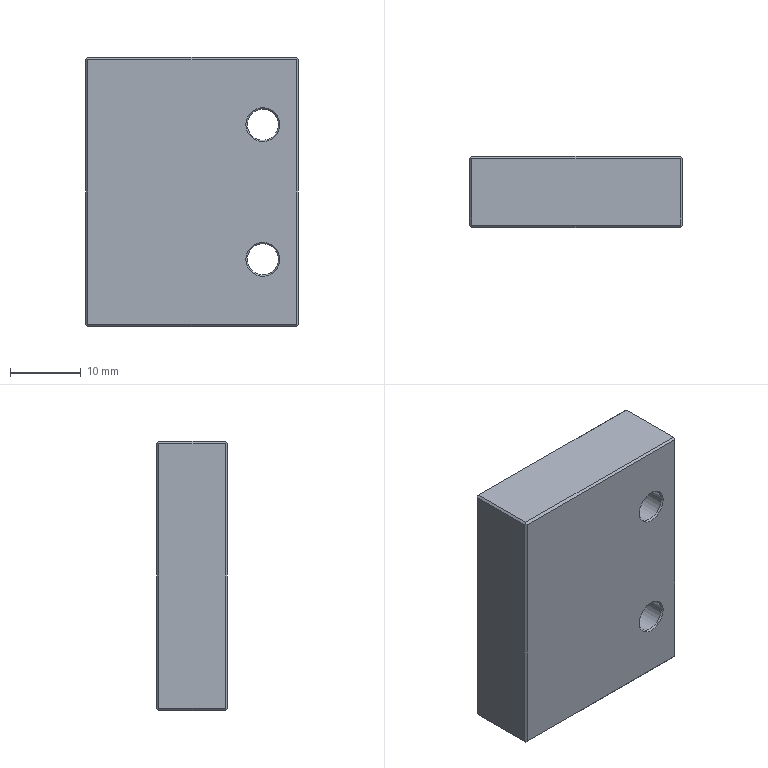Part | NX | 1 solid | 42 faces | box 30 x 10 x 38 mm | volume 10990 mm3 | plane 18 | cylinder 12 | cone 12 | commonest cylinder face diameters 2.5 x8 4.4 x4
STEP:
#1=CARTESIAN_POINT('',(-28.3,-35.,40.2));
#2=VERTEX_POINT('',#1);
#3=CARTESIAN_POINT('',(-28.3,-35.,2.8));
#4=VERTEX_POINT('',#3);
#5=CARTESIAN_POINT('',(-28.3,-35.,21.5));
#6=DIRECTION('',(0.,0.,-1.));
#7=VECTOR('',#6,1000.);
#8=LINE('',#5,#7);
#9=EDGE_CURVE('',#2,#4,#8,.T.);
#10=ORIENTED_EDGE('',*,*,#9,.F.);
#11=CARTESIAN_POINT('',(-57.7,-35.,40.2));
#12=VERTEX_POINT('',#11);
#13=CARTESIAN_POINT('',(-43.,-35.,40.2));
#14=DIRECTION('',(-1.,0.,0.));
#15=VECTOR('',#14,1000.);
#16=LINE('',#13,#15);
#17=EDGE_CURVE('',#2,#12,#16,.T.);
#18=ORIENTED_EDGE('',*,*,#17,.T.);
#19=CARTESIAN_POINT('',(-57.7,-35.,2.8));
#20=VERTEX_POINT('',#19);
#21=CARTESIAN_POINT('',(-57.7,-35.,21.5));
#22=DIRECTION('',(0.,0.,-1.));
#23=VECTOR('',#22,1000.);
#24=LINE('',#21,#23);
#25=EDGE_CURVE('',#12,#20,#24,.T.);
#26=ORIENTED_EDGE('',*,*,#25,.T.);
#27=CARTESIAN_POINT('',(-43.,-35.,2.8));
#28=DIRECTION('',(1.,0.,0.));
#29=VECTOR('',#28,1000.);
#30=LINE('',#27,#29);
#31=EDGE_CURVE('',#20,#4,#30,.T.);
#32=ORIENTED_EDGE('',*,*,#31,.T.);
#33=EDGE_LOOP('',(#10,#18,#26,#32));
#34=FACE_BOUND('',#33,.T.);
#35=CARTESIAN_POINT('',(-30.6,-35.,31.));
#36=VERTEX_POINT('',#35);
#37=CARTESIAN_POINT('',(-35.4,-35.,31.));
#38=VERTEX_POINT('',#37);
#39=CARTESIAN_POINT('',(-33.,-35.,31.));
#40=DIRECTION('',(0.,-1.,0.));
#41=DIRECTION('',(-1.,0.,0.));
#42=AXIS2_PLACEMENT_3D('',#39,#40,#41);
#43=CIRCLE('',#42,2.4);
#44=EDGE_CURVE('',#36,#38,#43,.T.);
#45=ORIENTED_EDGE('',*,*,#44,.F.);
#46=CARTESIAN_POINT('',(-33.,-35.,31.));
#47=DIRECTION('',(0.,-1.,0.));
#48=DIRECTION('',(-1.,0.,0.));
#49=AXIS2_PLACEMENT_3D('',#46,#47,#48);
#50=CIRCLE('',#49,2.4);
#51=EDGE_CURVE('',#38,#36,#50,.T.);
#52=ORIENTED_EDGE('',*,*,#51,.F.);
#53=EDGE_LOOP('',(#45,#52));
#54=FACE_BOUND('',#53,.T.);
#55=CARTESIAN_POINT('',(-30.6,-35.,12.));
#56=VERTEX_POINT('',#55);
#57=CARTESIAN_POINT('',(-35.4,-35.,12.));
#58=VERTEX_POINT('',#57);
#59=CARTESIAN_POINT('',(-33.,-35.,12.));
#60=DIRECTION('',(0.,-1.,0.));
#61=DIRECTION('',(-1.,0.,0.));
#62=AXIS2_PLACEMENT_3D('',#59,#60,#61);
#63=CIRCLE('',#62,2.4);
#64=EDGE_CURVE('',#56,#58,#63,.T.);
#65=ORIENTED_EDGE('',*,*,#64,.F.);
#66=CARTESIAN_POINT('',(-33.,-35.,12.));
#67=DIRECTION('',(0.,-1.,0.));
#68=DIRECTION('',(-1.,0.,0.));
#69=AXIS2_PLACEMENT_3D('',#66,#67,#68);
#70=CIRCLE('',#69,2.4);
#71=EDGE_CURVE('',#58,#56,#70,.T.);
#72=ORIENTED_EDGE('',*,*,#71,.F.);
#73=EDGE_LOOP('',(#65,#72));
#74=FACE_BOUND('',#73,.T.);
#75=CARTESIAN_POINT('',(0.,-35.,0.));
#76=DIRECTION('',(0.,1.,0.));
#77=DIRECTION('',(1.,0.,0.));
#78=AXIS2_PLACEMENT_3D('',#75,#76,#77);
#79=PLANE('',#78);
#80=ADVANCED_FACE('',(#34,#54,#74),#79,.F.);
#81=CARTESIAN_POINT('',(-58.,-25.3,2.8));
#82=VERTEX_POINT('',#81);
#83=CARTESIAN_POINT('',(-58.,-25.3,40.2));
#84=VERTEX_POINT('',#83);
#85=CARTESIAN_POINT('',(-58.,-25.3,21.5));
#86=DIRECTION('',(0.,0.,1.));
#87=VECTOR('',#86,1000.);
#88=LINE('',#85,#87);
#89=EDGE_CURVE('',#82,#84,#88,.T.);
#90=ORIENTED_EDGE('',*,*,#89,.F.);
#91=CARTESIAN_POINT('',(-58.,-34.7,2.8));
#92=VERTEX_POINT('',#91);
#93=CARTESIAN_POINT('',(-58.,-30.,2.8));
#94=DIRECTION('',(0.,1.,0.));
#95=VECTOR('',#94,1000.);
#96=LINE('',#93,#95);
#97=EDGE_CURVE('',#92,#82,#96,.T.);
#98=ORIENTED_EDGE('',*,*,#97,.F.);
#99=CARTESIAN_POINT('',(-58.,-34.7,40.2));
#100=VERTEX_POINT('',#99);
#101=CARTESIAN_POINT('',(-58.,-34.7,21.5));
#102=DIRECTION('',(0.,0.,-1.));
#103=VECTOR('',#102,1000.);
#104=LINE('',#101,#103);
#105=EDGE_CURVE('',#100,#92,#104,.T.);
#106=ORIENTED_EDGE('',*,*,#105,.F.);
#107=CARTESIAN_POINT('',(-58.,-30.,40.2));
#108=DIRECTION('',(0.,-1.,0.));
#109=VECTOR('',#108,1000.);
#110=LINE('',#107,#109);
#111=EDGE_CURVE('',#84,#100,#110,.T.);
#112=ORIENTED_EDGE('',*,*,#111,.F.);
#113=EDGE_LOOP('',(#90,#98,#106,#112));
#114=FACE_BOUND('',#113,.T.);
#115=CARTESIAN_POINT('',(-58.,0.,0.));
#116=DIRECTION('',(1.,0.,0.));
#117=DIRECTION('',(0.,1.,0.));
#118=AXIS2_PLACEMENT_3D('',#115,#116,#117);
#119=PLANE('',#118);
#120=ADVANCED_FACE('',(#114),#119,.F.);
#121=CARTESIAN_POINT('',(-28.3,-25.,2.8));
#122=VERTEX_POINT('',#121);
#123=CARTESIAN_POINT('',(-28.3,-25.,40.2));
#124=VERTEX_POINT('',#123);
#125=CARTESIAN_POINT('',(-28.3,-25.,21.5));
#126=DIRECTION('',(0.,0.,1.));
#127=VECTOR('',#126,1000.);
#128=LINE('',#125,#127);
#129=EDGE_CURVE('',#122,#124,#128,.T.);
#130=ORIENTED_EDGE('',*,*,#129,.F.);
#131=CARTESIAN_POINT('',(-57.7,-25.,2.8));
#132=VERTEX_POINT('',#131);
#133=CARTESIAN_POINT('',(-43.,-25.,2.8));
#134=DIRECTION('',(1.,0.,0.));
#135=VECTOR('',#134,1000.);
#136=LINE('',#133,#135);
#137=EDGE_CURVE('',#132,#122,#136,.T.);
#138=ORIENTED_EDGE('',*,*,#137,.F.);
#139=CARTESIAN_POINT('',(-57.7,-25.,40.2));
#140=VERTEX_POINT('',#139);
#141=CARTESIAN_POINT('',(-57.7,-25.,21.5));
#142=DIRECTION('',(0.,0.,1.));
#143=VECTOR('',#142,1000.);
#144=LINE('',#141,#143);
#145=EDGE_CURVE('',#132,#140,#144,.T.);
#146=ORIENTED_EDGE('',*,*,#145,.T.);
#147=CARTESIAN_POINT('',(-43.,-25.,40.2));
#148=DIRECTION('',(-1.,0.,0.));
#149=VECTOR('',#148,1000.);
#150=LINE('',#147,#149);
#151=EDGE_CURVE('',#124,#140,#150,.T.);
#152=ORIENTED_EDGE('',*,*,#151,.F.);
#153=EDGE_LOOP('',(#130,#138,#146,#152));
#154=FACE_BOUND('',#153,.T.);
#155=CARTESIAN_POINT('',(-30.8,-25.,12.));
#156=VERTEX_POINT('',#155);
#157=CARTESIAN_POINT('',(-35.2,-25.,12.));
#158=VERTEX_POINT('',#157);
#159=CARTESIAN_POINT('',(-33.,-25.,12.));
#160=DIRECTION('',(0.,-1.,0.));
#161=DIRECTION('',(-1.,0.,0.));
#162=AXIS2_PLACEMENT_3D('',#159,#160,#161);
#163=CIRCLE('',#162,2.2);
#164=EDGE_CURVE('',#156,#158,#163,.T.);
#165=ORIENTED_EDGE('',*,*,#164,.T.);
#166=CARTESIAN_POINT('',(-33.,-25.,12.));
#167=DIRECTION('',(0.,-1.,0.));
#168=DIRECTION('',(-1.,0.,0.));
#169=AXIS2_PLACEMENT_3D('',#166,#167,#168);
#170=CIRCLE('',#169,2.2);
#171=EDGE_CURVE('',#158,#156,#170,.T.);
#172=ORIENTED_EDGE('',*,*,#171,.T.);
#173=EDGE_LOOP('',(#165,#172));
#174=FACE_BOUND('',#173,.T.);
#175=CARTESIAN_POINT('',(-30.8,-25.,31.));
#176=VERTEX_POINT('',#175);
#177=CARTESIAN_POINT('',(-35.2,-25.,31.));
#178=VERTEX_POINT('',#177);
#179=CARTESIAN_POINT('',(-33.,-25.,31.));
#180=DIRECTION('',(0.,-1.,0.));
#181=DIRECTION('',(-1.,0.,0.));
#182=AXIS2_PLACEMENT_3D('',#179,#180,#181);
#183=CIRCLE('',#182,2.2);
#184=EDGE_CURVE('',#176,#178,#183,.T.);
#185=ORIENTED_EDGE('',*,*,#184,.T.);
#186=CARTESIAN_POINT('',(-33.,-25.,31.));
#187=DIRECTION('',(0.,-1.,0.));
#188=DIRECTION('',(-1.,0.,0.));
#189=AXIS2_PLACEMENT_3D('',#186,#187,#188);
#190=CIRCLE('',#189,2.2);
#191=EDGE_CURVE('',#178,#176,#190,.T.);
#192=ORIENTED_EDGE('',*,*,#191,.T.);
#193=EDGE_LOOP('',(#185,#192));
#194=FACE_BOUND('',#193,.T.);
#195=CARTESIAN_POINT('',(-8.5,-25.,1.2));
#196=DIRECTION('',(0.,-1.,0.));
#197=DIRECTION('',(-1.,0.,0.));
#198=AXIS2_PLACEMENT_3D('',#195,#196,#197);
#199=PLANE('',#198);
#200=ADVANCED_FACE('',(#154,#174,#194),#199,.F.);
#201=CARTESIAN_POINT('',(-28.3,-34.7,2.5));
#202=VERTEX_POINT('',#201);
#203=CARTESIAN_POINT('',(-28.3,-25.3,2.5));
#204=VERTEX_POINT('',#203);
#205=CARTESIAN_POINT('',(-28.3,-30.,2.5));
#206=DIRECTION('',(0.,1.,0.));
#207=VECTOR('',#206,1000.);
#208=LINE('',#205,#207);
#209=EDGE_CURVE('',#202,#204,#208,.T.);
#210=ORIENTED_EDGE('',*,*,#209,.F.);
#211=CARTESIAN_POINT('',(-57.7,-34.7,2.5));
#212=VERTEX_POINT('',#211);
#213=CARTESIAN_POINT('',(-43.,-34.7,2.5));
#214=DIRECTION('',(1.,0.,0.));
#215=VECTOR('',#214,1000.);
#216=LINE('',#213,#215);
#217=EDGE_CURVE('',#212,#202,#216,.T.);
#218=ORIENTED_EDGE('',*,*,#217,.F.);
#219=CARTESIAN_POINT('',(-57.7,-25.3,2.5));
#220=VERTEX_POINT('',#219);
#221=CARTESIAN_POINT('',(-57.7,-30.,2.5));
#222=DIRECTION('',(0.,1.,0.));
#223=VECTOR('',#222,1000.);
#224=LINE('',#221,#223);
#225=EDGE_CURVE('',#212,#220,#224,.T.);
#226=ORIENTED_EDGE('',*,*,#225,.T.);
#227=CARTESIAN_POINT('',(-43.,-25.3,2.5));
#228=DIRECTION('',(1.,0.,0.));
#229=VECTOR('',#228,1000.);
#230=LINE('',#227,#229);
#231=EDGE_CURVE('',#220,#204,#230,.T.);
#232=ORIENTED_EDGE('',*,*,#231,.T.);
#233=EDGE_LOOP('',(#210,#218,#226,#232));
#234=FACE_BOUND('',#233,.T.);
#235=CARTESIAN_POINT('',(-50.3,-31.,2.5));
#236=VERTEX_POINT('',#235);
#237=CARTESIAN_POINT('',(-53.7,-31.,2.5));
#238=VERTEX_POINT('',#237);
#239=CARTESIAN_POINT('',(-52.,-31.,2.5));
#240=DIRECTION('',(0.,0.,-1.));
#241=DIRECTION('',(-1.,0.,0.));
#242=AXIS2_PLACEMENT_3D('',#239,#240,#241);
#243=CIRCLE('',#242,1.7);
#244=EDGE_CURVE('',#236,#238,#243,.T.);
#245=ORIENTED_EDGE('',*,*,#244,.F.);
#246=CARTESIAN_POINT('',(-52.,-31.,2.5));
#247=DIRECTION('',(0.,0.,-1.));
#248=DIRECTION('',(-1.,0.,0.));
#249=AXIS2_PLACEMENT_3D('',#246,#247,#248);
#250=CIRCLE('',#249,1.7);
#251=EDGE_CURVE('',#238,#236,#250,.T.);
#252=ORIENTED_EDGE('',*,*,#251,.F.);
#253=EDGE_LOOP('',(#245,#252));
#254=FACE_BOUND('',#253,.T.);
#255=CARTESIAN_POINT('',(-43.3,-31.,2.5));
#256=VERTEX_POINT('',#255);
#257=CARTESIAN_POINT('',(-46.7,-31.,2.5));
#258=VERTEX_POINT('',#257);
#259=CARTESIAN_POINT('',(-45.,-31.,2.5));
#260=DIRECTION('',(0.,0.,-1.));
#261=DIRECTION('',(-1.,0.,0.));
#262=AXIS2_PLACEMENT_3D('',#259,#260,#261);
#263=CIRCLE('',#262,1.7);
#264=EDGE_CURVE('',#256,#258,#263,.T.);
#265=ORIENTED_EDGE('',*,*,#264,.F.);
#266=CARTESIAN_POINT('',(-45.,-31.,2.5));
#267=DIRECTION('',(0.,0.,-1.));
#268=DIRECTION('',(-1.,0.,0.));
#269=AXIS2_PLACEMENT_3D('',#266,#267,#268);
#270=CIRCLE('',#269,1.7);
#271=EDGE_CURVE('',#258,#256,#270,.T.);
#272=ORIENTED_EDGE('',*,*,#271,.F.);
#273=EDGE_LOOP('',(#265,#272));
#274=FACE_BOUND('',#273,.T.);
#275=CARTESIAN_POINT('',(-35.,0.,2.5));
#276=DIRECTION('',(0.,0.,1.));
#277=DIRECTION('',(1.,0.,0.));
#278=AXIS2_PLACEMENT_3D('',#275,#276,#277);
#279=PLANE('',#278);
#280=ADVANCED_FACE('',(#234,#254,#274),#279,.F.);
#281=CARTESIAN_POINT('',(-28.,-34.7,40.2));
#282=VERTEX_POINT('',#281);
#283=CARTESIAN_POINT('',(-28.,-25.3,40.2));
#284=VERTEX_POINT('',#283);
#285=CARTESIAN_POINT('',(-28.,-30.,40.2));
#286=DIRECTION('',(0.,1.,0.));
#287=VECTOR('',#286,1000.);
#288=LINE('',#285,#287);
#289=EDGE_CURVE('',#282,#284,#288,.T.);
#290=ORIENTED_EDGE('',*,*,#289,.F.);
#291=CARTESIAN_POINT('',(-28.,-34.7,2.8));
#292=VERTEX_POINT('',#291);
#293=CARTESIAN_POINT('',(-28.,-34.7,21.5));
#294=DIRECTION('',(0.,0.,-1.));
#295=VECTOR('',#294,1000.);
#296=LINE('',#293,#295);
#297=EDGE_CURVE('',#282,#292,#296,.T.);
#298=ORIENTED_EDGE('',*,*,#297,.T.);
#299=CARTESIAN_POINT('',(-28.,-25.3,2.8));
#300=VERTEX_POINT('',#299);
#301=CARTESIAN_POINT('',(-28.,-30.,2.8));
#302=DIRECTION('',(0.,1.,0.));
#303=VECTOR('',#302,1000.);
#304=LINE('',#301,#303);
#305=EDGE_CURVE('',#292,#300,#304,.T.);
#306=ORIENTED_EDGE('',*,*,#305,.T.);
#307=CARTESIAN_POINT('',(-28.,-25.3,21.5));
#308=DIRECTION('',(0.,0.,1.));
#309=VECTOR('',#308,1000.);
#310=LINE('',#307,#309);
#311=EDGE_CURVE('',#300,#284,#310,.T.);
#312=ORIENTED_EDGE('',*,*,#311,.T.);
#313=EDGE_LOOP('',(#290,#298,#306,#312));
#314=FACE_BOUND('',#313,.T.);
#315=CARTESIAN_POINT('',(-28.,-38.5,5.));
#316=DIRECTION('',(1.,0.,0.));
#317=DIRECTION('',(0.,1.,0.));
#318=AXIS2_PLACEMENT_3D('',#315,#316,#317);
#319=PLANE('',#318);
#320=ADVANCED_FACE('',(#314),#319,.T.);
#321=CARTESIAN_POINT('',(-57.7,-25.3,40.5));
#322=VERTEX_POINT('',#321);
#323=CARTESIAN_POINT('',(-57.7,-34.7,40.5));
#324=VERTEX_POINT('',#323);
#325=CARTESIAN_POINT('',(-57.7,-30.,40.5));
#326=DIRECTION('',(0.,-1.,0.));
#327=VECTOR('',#326,1000.);
#328=LINE('',#325,#327);
#329=EDGE_CURVE('',#322,#324,#328,.T.);
#330=ORIENTED_EDGE('',*,*,#329,.T.);
#331=CARTESIAN_POINT('',(-28.3,-34.7,40.5));
#332=VERTEX_POINT('',#331);
#333=CARTESIAN_POINT('',(-43.,-34.7,40.5));
#334=DIRECTION('',(-1.,0.,0.));
#335=VECTOR('',#334,1000.);
#336=LINE('',#333,#335);
#337=EDGE_CURVE('',#332,#324,#336,.T.);
#338=ORIENTED_EDGE('',*,*,#337,.F.);
#339=CARTESIAN_POINT('',(-28.3,-25.3,40.5));
#340=VERTEX_POINT('',#339);
#341=CARTESIAN_POINT('',(-28.3,-30.,40.5));
#342=DIRECTION('',(0.,1.,0.));
#343=VECTOR('',#342,1000.);
#344=LINE('',#341,#343);
#345=EDGE_CURVE('',#332,#340,#344,.T.);
#346=ORIENTED_EDGE('',*,*,#345,.T.);
#347=CARTESIAN_POINT('',(-43.,-25.3,40.5));
#348=DIRECTION('',(-1.,0.,0.));
#349=VECTOR('',#348,1000.);
#350=LINE('',#347,#349);
#351=EDGE_CURVE('',#340,#322,#350,.T.);
#352=ORIENTED_EDGE('',*,*,#351,.T.);
#353=EDGE_LOOP('',(#330,#338,#346,#352));
#354=FACE_BOUND('',#353,.T.);
#355=CARTESIAN_POINT('',(-20.5,7.5,40.5));
#356=DIRECTION('',(0.,0.,-1.));
#357=DIRECTION('',(0.,-1.,0.));
#358=AXIS2_PLACEMENT_3D('',#355,#356,#357);
#359=PLANE('',#358);
#360=ADVANCED_FACE('',(#354),#359,.F.);
#361=CARTESIAN_POINT('',(-43.75,-31.,2.76));
#362=VERTEX_POINT('',#361);
#363=CARTESIAN_POINT('',(-46.25,-31.,2.76));
#364=VERTEX_POINT('',#363);
#365=CARTESIAN_POINT('',(-45.,-31.,2.76));
#366=DIRECTION('',(0.,0.,-1.));
#367=DIRECTION('',(-1.,0.,0.));
#368=AXIS2_PLACEMENT_3D('',#365,#366,#367);
#369=CIRCLE('',#368,1.25);
#370=EDGE_CURVE('',#362,#364,#369,.T.);
#371=ORIENTED_EDGE('',*,*,#370,.T.);
#372=CARTESIAN_POINT('',(-46.25,-31.,8.5));
#373=VERTEX_POINT('',#372);
#374=CARTESIAN_POINT('',(-46.25,-31.,2.5));
#375=DIRECTION('',(0.,0.,-1.));
#376=VECTOR('',#375,1000.);
#377=LINE('',#374,#376);
#378=EDGE_CURVE('',#364,#373,#377,.F.);
#379=ORIENTED_EDGE('',*,*,#378,.T.);
#380=CARTESIAN_POINT('',(-43.75,-31.,8.5));
#381=VERTEX_POINT('',#380);
#382=CARTESIAN_POINT('',(-45.,-31.,8.5));
#383=DIRECTION('',(0.,0.,-1.));
#384=DIRECTION('',(-1.,0.,0.));
#385=AXIS2_PLACEMENT_3D('',#382,#383,#384);
#386=CIRCLE('',#385,1.25);
#387=EDGE_CURVE('',#381,#373,#386,.T.);
#388=ORIENTED_EDGE('',*,*,#387,.F.);
#389=CARTESIAN_POINT('',(-43.75,-31.,2.5));
#390=DIRECTION('',(0.,0.,-1.));
#391=VECTOR('',#390,1000.);
#392=LINE('',#389,#391);
#393=EDGE_CURVE('',#362,#381,#392,.F.);
#394=ORIENTED_EDGE('',*,*,#393,.F.);
#395=EDGE_LOOP('',(#371,#379,#388,#394));
#396=FACE_BOUND('',#395,.T.);
#397=CARTESIAN_POINT('',(-45.,-31.,2.5));
#398=DIRECTION('',(0.,0.,-1.));
#399=DIRECTION('',(-1.,0.,0.));
#400=AXIS2_PLACEMENT_3D('',#397,#398,#399);
#401=CYLINDRICAL_SURFACE('',#400,1.25);
#402=ADVANCED_FACE('',(#396),#401,.F.);
#403=ORIENTED_EDGE('',*,*,#387,.T.);
#404=CARTESIAN_POINT('',(-46.25,-31.,11.5));
#405=VERTEX_POINT('',#404);
#406=CARTESIAN_POINT('',(-46.25,-31.,2.5));
#407=DIRECTION('',(0.,0.,-1.));
#408=VECTOR('',#407,1000.);
#409=LINE('',#406,#408);
#410=EDGE_CURVE('',#373,#405,#409,.F.);
#411=ORIENTED_EDGE('',*,*,#410,.T.);
#412=CARTESIAN_POINT('',(-43.75,-31.,11.5));
#413=VERTEX_POINT('',#412);
#414=CARTESIAN_POINT('',(-45.,-31.,11.5));
#415=DIRECTION('',(0.,0.,-1.));
#416=DIRECTION('',(-1.,0.,0.));
#417=AXIS2_PLACEMENT_3D('',#414,#415,#416);
#418=CIRCLE('',#417,1.25);
#419=EDGE_CURVE('',#413,#405,#418,.T.);
#420=ORIENTED_EDGE('',*,*,#419,.F.);
#421=CARTESIAN_POINT('',(-43.75,-31.,2.5));
#422=DIRECTION('',(0.,0.,-1.));
#423=VECTOR('',#422,1000.);
#424=LINE('',#421,#423);
#425=EDGE_CURVE('',#381,#413,#424,.F.);
#426=ORIENTED_EDGE('',*,*,#425,.F.);
#427=EDGE_LOOP('',(#403,#411,#420,#426));
#428=FACE_BOUND('',#427,.T.);
#429=CARTESIAN_POINT('',(-45.,-31.,2.5));
#430=DIRECTION('',(0.,0.,-1.));
#431=DIRECTION('',(-1.,0.,0.));
#432=AXIS2_PLACEMENT_3D('',#429,#430,#431);
#433=CYLINDRICAL_SURFACE('',#432,1.25);
#434=ADVANCED_FACE('',(#428),#433,.F.);
#435=ORIENTED_EDGE('',*,*,#419,.T.);
#436=CARTESIAN_POINT('',(-45.,-31.,12.251));
#437=VERTEX_POINT('',#436);
#438=CARTESIAN_POINT('',(-46.25,-31.,11.5));
#439=DIRECTION('',(-0.8572,0.,-0.515));
#440=VECTOR('',#439,1000.);
#441=LINE('',#438,#440);
#442=EDGE_CURVE('',#437,#405,#441,.T.);
#443=ORIENTED_EDGE('',*,*,#442,.F.);
#444=CARTESIAN_POINT('',(-43.75,-31.,11.5));
#445=DIRECTION('',(0.8572,0.,-0.515));
#446=VECTOR('',#445,1000.);
#447=LINE('',#444,#446);
#448=EDGE_CURVE('',#437,#413,#447,.T.);
#449=ORIENTED_EDGE('',*,*,#448,.T.);
#450=EDGE_LOOP('',(#435,#443,#449));
#451=FACE_BOUND('',#450,.T.);
#452=CARTESIAN_POINT('',(-45.,-31.,11.5));
#453=DIRECTION('',(0.,0.,-1.));
#454=DIRECTION('',(-1.,0.,0.));
#455=AXIS2_PLACEMENT_3D('',#452,#453,#454);
#456=CONICAL_SURFACE('',#455,1.25,1.03);
#457=ADVANCED_FACE('',(#451),#456,.F.);
#458=CARTESIAN_POINT('',(-30.8,-34.8,31.));
#459=VERTEX_POINT('',#458);
#460=CARTESIAN_POINT('',(-35.2,-34.8,31.));
#461=VERTEX_POINT('',#460);
#462=CARTESIAN_POINT('',(-33.,-34.8,31.));
#463=DIRECTION('',(0.,-1.,0.));
#464=DIRECTION('',(-1.,0.,0.));
#465=AXIS2_PLACEMENT_3D('',#462,#463,#464);
#466=CIRCLE('',#465,2.2);
#467=EDGE_CURVE('',#459,#461,#466,.T.);
#468=ORIENTED_EDGE('',*,*,#467,.T.);
#469=CARTESIAN_POINT('',(-35.2,-35.,31.));
#470=DIRECTION('',(0.,-1.,0.));
#471=VECTOR('',#470,1000.);
#472=LINE('',#469,#471);
#473=EDGE_CURVE('',#461,#178,#472,.F.);
#474=ORIENTED_EDGE('',*,*,#473,.T.);
#475=ORIENTED_EDGE('',*,*,#184,.F.);
#476=CARTESIAN_POINT('',(-30.8,-35.,31.));
#477=DIRECTION('',(0.,-1.,0.));
#478=VECTOR('',#477,1000.);
#479=LINE('',#476,#478);
#480=EDGE_CURVE('',#459,#176,#479,.F.);
#481=ORIENTED_EDGE('',*,*,#480,.F.);
#482=EDGE_LOOP('',(#468,#474,#475,#481));
#483=FACE_BOUND('',#482,.T.);
#484=CARTESIAN_POINT('',(-33.,-35.,31.));
#485=DIRECTION('',(0.,-1.,0.));
#486=DIRECTION('',(-1.,0.,0.));
#487=AXIS2_PLACEMENT_3D('',#484,#485,#486);
#488=CYLINDRICAL_SURFACE('',#487,2.2);
#489=ADVANCED_FACE('',(#483),#488,.F.);
#490=CARTESIAN_POINT('',(-50.75,-31.,2.76));
#491=VERTEX_POINT('',#490);
#492=CARTESIAN_POINT('',(-53.25,-31.,2.76));
#493=VERTEX_POINT('',#492);
#494=CARTESIAN_POINT('',(-52.,-31.,2.76));
#495=DIRECTION('',(0.,0.,-1.));
#496=DIRECTION('',(-1.,0.,0.));
#497=AXIS2_PLACEMENT_3D('',#494,#495,#496);
#498=CIRCLE('',#497,1.25);
#499=EDGE_CURVE('',#491,#493,#498,.T.);
#500=ORIENTED_EDGE('',*,*,#499,.T.);
#501=CARTESIAN_POINT('',(-53.25,-31.,8.5));
#502=VERTEX_POINT('',#501);
#503=CARTESIAN_POINT('',(-53.25,-31.,2.5));
#504=DIRECTION('',(0.,0.,-1.));
#505=VECTOR('',#504,1000.);
#506=LINE('',#503,#505);
#507=EDGE_CURVE('',#493,#502,#506,.F.);
#508=ORIENTED_EDGE('',*,*,#507,.T.);
#509=CARTESIAN_POINT('',(-50.75,-31.,8.5));
#510=VERTEX_POINT('',#509);
#511=CARTESIAN_POINT('',(-52.,-31.,8.5));
#512=DIRECTION('',(0.,0.,-1.));
#513=DIRECTION('',(-1.,0.,0.));
#514=AXIS2_PLACEMENT_3D('',#511,#512,#513);
#515=CIRCLE('',#514,1.25);
#516=EDGE_CURVE('',#510,#502,#515,.T.);
#517=ORIENTED_EDGE('',*,*,#516,.F.);
#518=CARTESIAN_POINT('',(-50.75,-31.,2.5));
#519=DIRECTION('',(0.,0.,-1.));
#520=VECTOR('',#519,1000.);
#521=LINE('',#518,#520);
#522=EDGE_CURVE('',#491,#510,#521,.F.);
#523=ORIENTED_EDGE('',*,*,#522,.F.);
#524=EDGE_LOOP('',(#500,#508,#517,#523));
#525=FACE_BOUND('',#524,.T.);
#526=CARTESIAN_POINT('',(-52.,-31.,2.5));
#527=DIRECTION('',(0.,0.,-1.));
#528=DIRECTION('',(-1.,0.,0.));
#529=AXIS2_PLACEMENT_3D('',#526,#527,#528);
#530=CYLINDRICAL_SURFACE('',#529,1.25);
#531=ADVANCED_FACE('',(#525),#530,.F.);
#532=ORIENTED_EDGE('',*,*,#516,.T.);
#533=CARTESIAN_POINT('',(-53.25,-31.,11.5));
#534=VERTEX_POINT('',#533);
#535=CARTESIAN_POINT('',(-53.25,-31.,2.5));
#536=DIRECTION('',(0.,0.,-1.));
#537=VECTOR('',#536,1000.);
#538=LINE('',#535,#537);
#539=EDGE_CURVE('',#502,#534,#538,.F.);
#540=ORIENTED_EDGE('',*,*,#539,.T.);
#541=CARTESIAN_POINT('',(-50.75,-31.,11.5));
#542=VERTEX_POINT('',#541);
#543=CARTESIAN_POINT('',(-52.,-31.,11.5));
#544=DIRECTION('',(0.,0.,-1.));
#545=DIRECTION('',(-1.,0.,0.));
#546=AXIS2_PLACEMENT_3D('',#543,#544,#545);
#547=CIRCLE('',#546,1.25);
#548=EDGE_CURVE('',#542,#534,#547,.T.);
#549=ORIENTED_EDGE('',*,*,#548,.F.);
#550=CARTESIAN_POINT('',(-50.75,-31.,2.5));
#551=DIRECTION('',(0.,0.,-1.));
#552=VECTOR('',#551,1000.);
#553=LINE('',#550,#552);
#554=EDGE_CURVE('',#510,#542,#553,.F.);
#555=ORIENTED_EDGE('',*,*,#554,.F.);
#556=EDGE_LOOP('',(#532,#540,#549,#555));
#557=FACE_BOUND('',#556,.T.);
#558=CARTESIAN_POINT('',(-52.,-31.,2.5));
#559=DIRECTION('',(0.,0.,-1.));
#560=DIRECTION('',(-1.,0.,0.));
#561=AXIS2_PLACEMENT_3D('',#558,#559,#560);
#562=CYLINDRICAL_SURFACE('',#561,1.25);
#563=ADVANCED_FACE('',(#557),#562,.F.);
#564=ORIENTED_EDGE('',*,*,#548,.T.);
#565=CARTESIAN_POINT('',(-52.,-31.,12.251));
#566=VERTEX_POINT('',#565);
#567=CARTESIAN_POINT('',(-53.25,-31.,11.5));
#568=DIRECTION('',(-0.8572,0.,-0.515));
#569=VECTOR('',#568,1000.);
#570=LINE('',#567,#569);
#571=EDGE_CURVE('',#566,#534,#570,.T.);
#572=ORIENTED_EDGE('',*,*,#571,.F.);
#573=CARTESIAN_POINT('',(-50.75,-31.,11.5));
#574=DIRECTION('',(0.8572,0.,-0.515));
#575=VECTOR('',#574,1000.);
#576=LINE('',#573,#575);
#577=EDGE_CURVE('',#566,#542,#576,.T.);
#578=ORIENTED_EDGE('',*,*,#577,.T.);
#579=EDGE_LOOP('',(#564,#572,#578));
#580=FACE_BOUND('',#579,.T.);
#581=CARTESIAN_POINT('',(-52.,-31.,11.5));
#582=DIRECTION('',(0.,0.,-1.));
#583=DIRECTION('',(-1.,0.,0.));
#584=AXIS2_PLACEMENT_3D('',#581,#582,#583);
#585=CONICAL_SURFACE('',#584,1.25,1.03);
#586=ADVANCED_FACE('',(#580),#585,.F.);
#587=CARTESIAN_POINT('',(-30.8,-34.8,12.));
#588=VERTEX_POINT('',#587);
#589=CARTESIAN_POINT('',(-35.2,-34.8,12.));
#590=VERTEX_POINT('',#589);
#591=CARTESIAN_POINT('',(-33.,-34.8,12.));
#592=DIRECTION('',(0.,-1.,0.));
#593=DIRECTION('',(-1.,0.,0.));
#594=AXIS2_PLACEMENT_3D('',#591,#592,#593);
#595=CIRCLE('',#594,2.2);
#596=EDGE_CURVE('',#588,#590,#595,.T.);
#597=ORIENTED_EDGE('',*,*,#596,.T.);
#598=CARTESIAN_POINT('',(-35.2,-35.,12.));
#599=DIRECTION('',(0.,-1.,0.));
#600=VECTOR('',#599,1000.);
#601=LINE('',#598,#600);
#602=EDGE_CURVE('',#590,#158,#601,.F.);
#603=ORIENTED_EDGE('',*,*,#602,.T.);
#604=ORIENTED_EDGE('',*,*,#164,.F.);
#605=CARTESIAN_POINT('',(-30.8,-35.,12.));
#606=DIRECTION('',(0.,-1.,0.));
#607=VECTOR('',#606,1000.);
#608=LINE('',#605,#607);
#609=EDGE_CURVE('',#588,#156,#608,.F.);
#610=ORIENTED_EDGE('',*,*,#609,.F.);
#611=EDGE_LOOP('',(#597,#603,#604,#610));
#612=FACE_BOUND('',#611,.T.);
#613=CARTESIAN_POINT('',(-33.,-35.,12.));
#614=DIRECTION('',(0.,-1.,0.));
#615=DIRECTION('',(-1.,0.,0.));
#616=AXIS2_PLACEMENT_3D('',#613,#614,#615);
#617=CYLINDRICAL_SURFACE('',#616,2.2);
#618=ADVANCED_FACE('',(#612),#617,.F.);
#619=ORIENTED_EDGE('',*,*,#370,.F.);
#620=CARTESIAN_POINT('',(-43.75,-31.,2.76));
#621=DIRECTION('',(0.866,0.,-0.5));
#622=VECTOR('',#621,1000.);
#623=LINE('',#620,#622);
#624=EDGE_CURVE('',#256,#362,#623,.F.);
#625=ORIENTED_EDGE('',*,*,#624,.F.);
#626=ORIENTED_EDGE('',*,*,#264,.T.);
#627=CARTESIAN_POINT('',(-46.25,-31.,2.76));
#628=DIRECTION('',(-0.866,0.,-0.5));
#629=VECTOR('',#628,1000.);
#630=LINE('',#627,#629);
#631=EDGE_CURVE('',#258,#364,#630,.F.);
#632=ORIENTED_EDGE('',*,*,#631,.T.);
#633=EDGE_LOOP('',(#619,#625,#626,#632));
#634=FACE_BOUND('',#633,.T.);
#635=CARTESIAN_POINT('',(-45.,-31.,2.76));
#636=DIRECTION('',(0.,0.,-1.));
#637=DIRECTION('',(-1.,0.,0.));
#638=AXIS2_PLACEMENT_3D('',#635,#636,#637);
#639=CONICAL_SURFACE('',#638,1.25,1.047);
#640=ADVANCED_FACE('',(#634),#639,.F.);
#641=ORIENTED_EDGE('',*,*,#499,.F.);
#642=CARTESIAN_POINT('',(-50.75,-31.,2.76));
#643=DIRECTION('',(0.866,0.,-0.5));
#644=VECTOR('',#643,1000.);
#645=LINE('',#642,#644);
#646=EDGE_CURVE('',#236,#491,#645,.F.);
#647=ORIENTED_EDGE('',*,*,#646,.F.);
#648=ORIENTED_EDGE('',*,*,#244,.T.);
#649=CARTESIAN_POINT('',(-53.25,-31.,2.76));
#650=DIRECTION('',(-0.866,0.,-0.5));
#651=VECTOR('',#650,1000.);
#652=LINE('',#649,#651);
#653=EDGE_CURVE('',#238,#493,#652,.F.);
#654=ORIENTED_EDGE('',*,*,#653,.T.);
#655=EDGE_LOOP('',(#641,#647,#648,#654));
#656=FACE_BOUND('',#655,.T.);
#657=CARTESIAN_POINT('',(-52.,-31.,2.76));
#658=DIRECTION('',(0.,0.,-1.));
#659=DIRECTION('',(-1.,0.,0.));
#660=AXIS2_PLACEMENT_3D('',#657,#658,#659);
#661=CONICAL_SURFACE('',#660,1.25,1.047);
#662=ADVANCED_FACE('',(#656),#661,.F.);
#663=ORIENTED_EDGE('',*,*,#596,.F.);
#664=CARTESIAN_POINT('',(-30.8,-34.8,12.));
#665=DIRECTION('',(0.7071,-0.7071,0.));
#666=VECTOR('',#665,1000.);
#667=LINE('',#664,#666);
#668=EDGE_CURVE('',#56,#588,#667,.F.);
#669=ORIENTED_EDGE('',*,*,#668,.F.);
#670=ORIENTED_EDGE('',*,*,#64,.T.);
#671=CARTESIAN_POINT('',(-35.2,-34.8,12.));
#672=DIRECTION('',(-0.7071,-0.7071,0.));
#673=VECTOR('',#672,1000.);
#674=LINE('',#671,#673);
#675=EDGE_CURVE('',#58,#590,#674,.F.);
#676=ORIENTED_EDGE('',*,*,#675,.T.);
#677=EDGE_LOOP('',(#663,#669,#670,#676));
#678=FACE_BOUND('',#677,.T.);
#679=CARTESIAN_POINT('',(-33.,-34.8,12.));
#680=DIRECTION('',(0.,-1.,0.));
#681=DIRECTION('',(-1.,0.,0.));
#682=AXIS2_PLACEMENT_3D('',#679,#680,#681);
#683=CONICAL_SURFACE('',#682,2.2,0.7854);
#684=ADVANCED_FACE('',(#678),#683,.F.);
#685=ORIENTED_EDGE('',*,*,#467,.F.);
#686=CARTESIAN_POINT('',(-30.8,-34.8,31.));
#687=DIRECTION('',(0.7071,-0.7071,0.));
#688=VECTOR('',#687,1000.);
#689=LINE('',#686,#688);
#690=EDGE_CURVE('',#36,#459,#689,.F.);
#691=ORIENTED_EDGE('',*,*,#690,.F.);
#692=ORIENTED_EDGE('',*,*,#44,.T.);
#693=CARTESIAN_POINT('',(-35.2,-34.8,31.));
#694=DIRECTION('',(-0.7071,-0.7071,0.));
#695=VECTOR('',#694,1000.);
#696=LINE('',#693,#695);
#697=EDGE_CURVE('',#38,#461,#696,.F.);
#698=ORIENTED_EDGE('',*,*,#697,.T.);
#699=EDGE_LOOP('',(#685,#691,#692,#698));
#700=FACE_BOUND('',#699,.T.);
#701=CARTESIAN_POINT('',(-33.,-34.8,31.));
#702=DIRECTION('',(0.,-1.,0.));
#703=DIRECTION('',(-1.,0.,0.));
#704=AXIS2_PLACEMENT_3D('',#701,#702,#703);
#705=CONICAL_SURFACE('',#704,2.2,0.7854);
#706=ADVANCED_FACE('',(#700),#705,.F.);
#707=ORIENTED_EDGE('',*,*,#145,.F.);
#708=CARTESIAN_POINT('',(-57.85,-25.15,2.65));
#709=VERTEX_POINT('',#708);
#710=CARTESIAN_POINT('',(0.,32.7,60.5));
#711=DIRECTION('',(-0.5774,-0.5774,-0.5774));
#712=VECTOR('',#711,1000.);
#713=LINE('',#710,#712);
#714=EDGE_CURVE('',#132,#709,#713,.T.);
#715=ORIENTED_EDGE('',*,*,#714,.T.);
#716=CARTESIAN_POINT('',(-55.2,-22.5,0.));
#717=DIRECTION('',(-0.5774,-0.5774,0.5774));
#718=VECTOR('',#717,1000.);
#719=LINE('',#716,#718);
#720=EDGE_CURVE('',#709,#82,#719,.T.);
#721=ORIENTED_EDGE('',*,*,#720,.T.);
#722=ORIENTED_EDGE('',*,*,#89,.T.);
#723=CARTESIAN_POINT('',(-57.85,-25.15,40.35));
#724=VERTEX_POINT('',#723);
#725=CARTESIAN_POINT('',(-98.2,-65.5,0.));
#726=DIRECTION('',(0.5774,0.5774,0.5774));
#727=VECTOR('',#726,1000.);
#728=LINE('',#725,#727);
#729=EDGE_CURVE('',#84,#724,#728,.T.);
#730=ORIENTED_EDGE('',*,*,#729,.T.);
#731=CARTESIAN_POINT('',(0.,32.7,-17.5));
#732=DIRECTION('',(0.5774,0.5774,-0.5774));
#733=VECTOR('',#732,1000.);
#734=LINE('',#731,#733);
#735=EDGE_CURVE('',#724,#140,#734,.T.);
#736=ORIENTED_EDGE('',*,*,#735,.T.);
#737=EDGE_LOOP('',(#707,#715,#721,#722,#730,#736));
#738=FACE_BOUND('',#737,.T.);
#739=CARTESIAN_POINT('',(-57.85,-25.15,21.5));
#740=DIRECTION('',(-0.7071,0.7071,0.));
#741=DIRECTION('',(0.,0.,1.));
#742=AXIS2_PLACEMENT_3D('',#739,#740,#741);
#743=PLANE('',#742);
#744=ADVANCED_FACE('',(#738),#743,.T.);
#745=ORIENTED_EDGE('',*,*,#231,.F.);
#746=CARTESIAN_POINT('',(-83.,0.,27.8));
#747=DIRECTION('',(-0.5774,0.5774,0.5774));
#748=VECTOR('',#747,1000.);
#749=LINE('',#746,#748);
#750=EDGE_CURVE('',#220,#709,#749,.T.);
#751=ORIENTED_EDGE('',*,*,#750,.T.);
#752=ORIENTED_EDGE('',*,*,#714,.F.);
#753=ORIENTED_EDGE('',*,*,#137,.T.);
#754=CARTESIAN_POINT('',(-28.15,-25.15,2.65));
#755=VERTEX_POINT('',#754);
#756=CARTESIAN_POINT('',(-53.3,0.,27.8));
#757=DIRECTION('',(-0.5774,0.5774,0.5774));
#758=VECTOR('',#757,1000.);
#759=LINE('',#756,#758);
#760=EDGE_CURVE('',#755,#122,#759,.T.);
#761=ORIENTED_EDGE('',*,*,#760,.F.);
#762=CARTESIAN_POINT('',(0.,3.,30.8));
#763=DIRECTION('',(0.5774,0.5774,0.5774));
#764=VECTOR('',#763,1000.);
#765=LINE('',#762,#764);
#766=EDGE_CURVE('',#204,#755,#765,.T.);
#767=ORIENTED_EDGE('',*,*,#766,.F.);
#768=EDGE_LOOP('',(#745,#751,#752,#753,#761,#767));
#769=FACE_BOUND('',#768,.T.);
#770=CARTESIAN_POINT('',(-43.,-25.15,2.65));
#771=DIRECTION('',(0.,0.7071,-0.7071));
#772=DIRECTION('',(-1.,0.,0.));
#773=AXIS2_PLACEMENT_3D('',#770,#771,#772);
#774=PLANE('',#773);
#775=ADVANCED_FACE('',(#769),#774,.T.);
#776=ORIENTED_EDGE('',*,*,#225,.F.);
#777=CARTESIAN_POINT('',(-57.85,-34.85,2.65));
#778=VERTEX_POINT('',#777);
#779=CARTESIAN_POINT('',(-55.2,-32.2,0.));
#780=DIRECTION('',(-0.5774,-0.5774,0.5774));
#781=VECTOR('',#780,1000.);
#782=LINE('',#779,#781);
#783=EDGE_CURVE('',#212,#778,#782,.T.);
#784=ORIENTED_EDGE('',*,*,#783,.T.);
#785=CARTESIAN_POINT('',(-55.2,-37.5,0.));
#786=DIRECTION('',(-0.5774,0.5774,0.5774));
#787=VECTOR('',#786,1000.);
#788=LINE('',#785,#787);
#789=EDGE_CURVE('',#778,#92,#788,.T.);
#790=ORIENTED_EDGE('',*,*,#789,.T.);
#791=ORIENTED_EDGE('',*,*,#97,.T.);
#792=ORIENTED_EDGE('',*,*,#720,.F.);
#793=ORIENTED_EDGE('',*,*,#750,.F.);
#794=EDGE_LOOP('',(#776,#784,#790,#791,#792,#793));
#795=FACE_BOUND('',#794,.T.);
#796=CARTESIAN_POINT('',(-57.85,-30.,2.65));
#797=DIRECTION('',(-0.7071,0.,-0.7071));
#798=DIRECTION('',(-0.7071,0.,0.7071));
#799=AXIS2_PLACEMENT_3D('',#796,#797,#798);
#800=PLANE('',#799);
#801=ADVANCED_FACE('',(#795),#800,.T.);
#802=ORIENTED_EDGE('',*,*,#31,.F.);
#803=CARTESIAN_POINT('',(0.,-92.7,60.5));
#804=DIRECTION('',(-0.5774,0.5774,-0.5774));
#805=VECTOR('',#804,1000.);
#806=LINE('',#803,#805);
#807=EDGE_CURVE('',#20,#778,#806,.T.);
#808=ORIENTED_EDGE('',*,*,#807,.T.);
#809=ORIENTED_EDGE('',*,*,#783,.F.);
#810=ORIENTED_EDGE('',*,*,#217,.T.);
#811=CARTESIAN_POINT('',(-28.15,-34.85,2.65));
#812=VERTEX_POINT('',#811);
#813=CARTESIAN_POINT('',(0.,-63.,30.8));
#814=DIRECTION('',(-0.5774,0.5774,-0.5774));
#815=VECTOR('',#814,1000.);
#816=LINE('',#813,#815);
#817=EDGE_CURVE('',#812,#202,#816,.T.);
#818=ORIENTED_EDGE('',*,*,#817,.F.);
#819=CARTESIAN_POINT('',(0.,-6.7,-25.5));
#820=DIRECTION('',(0.5774,0.5774,-0.5774));
#821=VECTOR('',#820,1000.);
#822=LINE('',#819,#821);
#823=EDGE_CURVE('',#4,#812,#822,.T.);
#824=ORIENTED_EDGE('',*,*,#823,.F.);
#825=EDGE_LOOP('',(#802,#808,#809,#810,#818,#824));
#826=FACE_BOUND('',#825,.T.);
#827=CARTESIAN_POINT('',(-43.,-34.85,2.65));
#828=DIRECTION('',(0.,-0.7071,-0.7071));
#829=DIRECTION('',(0.,0.7071,-0.7071));
#830=AXIS2_PLACEMENT_3D('',#827,#828,#829);
#831=PLANE('',#830);
#832=ADVANCED_FACE('',(#826),#831,.T.);
#833=ORIENTED_EDGE('',*,*,#25,.F.);
#834=CARTESIAN_POINT('',(-57.85,-34.85,40.35));
#835=VERTEX_POINT('',#834);
#836=CARTESIAN_POINT('',(0.,-92.7,-17.5));
#837=DIRECTION('',(-0.5774,0.5774,0.5774));
#838=VECTOR('',#837,1000.);
#839=LINE('',#836,#838);
#840=EDGE_CURVE('',#12,#835,#839,.T.);
#841=ORIENTED_EDGE('',*,*,#840,.T.);
#842=CARTESIAN_POINT('',(-98.2,5.5,0.));
#843=DIRECTION('',(-0.5774,0.5774,-0.5774));
#844=VECTOR('',#843,1000.);
#845=LINE('',#842,#844);
#846=EDGE_CURVE('',#835,#100,#845,.T.);
#847=ORIENTED_EDGE('',*,*,#846,.T.);
#848=ORIENTED_EDGE('',*,*,#105,.T.);
#849=ORIENTED_EDGE('',*,*,#789,.F.);
#850=ORIENTED_EDGE('',*,*,#807,.F.);
#851=EDGE_LOOP('',(#833,#841,#847,#848,#849,#850));
#852=FACE_BOUND('',#851,.T.);
#853=CARTESIAN_POINT('',(-57.85,-34.85,21.5));
#854=DIRECTION('',(-0.7071,-0.7071,0.));
#855=DIRECTION('',(-0.7071,0.7071,0.));
#856=AXIS2_PLACEMENT_3D('',#853,#854,#855);
#857=PLANE('',#856);
#858=ADVANCED_FACE('',(#852),#857,.T.);
#859=ORIENTED_EDGE('',*,*,#17,.F.);
#860=CARTESIAN_POINT('',(-28.15,-34.85,40.35));
#861=VERTEX_POINT('',#860);
#862=CARTESIAN_POINT('',(0.,-6.7,68.5));
#863=DIRECTION('',(-0.5774,-0.5774,-0.5774));
#864=VECTOR('',#863,1000.);
#865=LINE('',#862,#864);
#866=EDGE_CURVE('',#861,#2,#865,.T.);
#867=ORIENTED_EDGE('',*,*,#866,.F.);
#868=CARTESIAN_POINT('',(0.,-63.,12.2));
#869=DIRECTION('',(0.5774,-0.5774,-0.5774));
#870=VECTOR('',#869,1000.);
#871=LINE('',#868,#870);
#872=EDGE_CURVE('',#332,#861,#871,.T.);
#873=ORIENTED_EDGE('',*,*,#872,.F.);
#874=ORIENTED_EDGE('',*,*,#337,.T.);
#875=CARTESIAN_POINT('',(-98.2,-75.2,0.));
#876=DIRECTION('',(-0.5774,-0.5774,-0.5774));
#877=VECTOR('',#876,1000.);
#878=LINE('',#875,#877);
#879=EDGE_CURVE('',#324,#835,#878,.T.);
#880=ORIENTED_EDGE('',*,*,#879,.T.);
#881=ORIENTED_EDGE('',*,*,#840,.F.);
#882=EDGE_LOOP('',(#859,#867,#873,#874,#880,#881));
#883=FACE_BOUND('',#882,.T.);
#884=CARTESIAN_POINT('',(-43.,-34.85,40.35));
#885=DIRECTION('',(0.,-0.7071,0.7071));
#886=DIRECTION('',(-1.,0.,0.));
#887=AXIS2_PLACEMENT_3D('',#884,#885,#886);
#888=PLANE('',#887);
#889=ADVANCED_FACE('',(#883),#888,.T.);
#890=ORIENTED_EDGE('',*,*,#9,.T.);
#891=ORIENTED_EDGE('',*,*,#823,.T.);
#892=CARTESIAN_POINT('',(0.,-6.7,30.8));
#893=DIRECTION('',(0.5774,0.5774,0.5774));
#894=VECTOR('',#893,1000.);
#895=LINE('',#892,#894);
#896=EDGE_CURVE('',#812,#292,#895,.T.);
#897=ORIENTED_EDGE('',*,*,#896,.T.);
#898=ORIENTED_EDGE('',*,*,#297,.F.);
#899=CARTESIAN_POINT('',(0.,-6.7,12.2));
#900=DIRECTION('',(-0.5774,-0.5774,0.5774));
#901=VECTOR('',#900,1000.);
#902=LINE('',#899,#901);
#903=EDGE_CURVE('',#282,#861,#902,.T.);
#904=ORIENTED_EDGE('',*,*,#903,.T.);
#905=ORIENTED_EDGE('',*,*,#866,.T.);
#906=EDGE_LOOP('',(#890,#891,#897,#898,#904,#905));
#907=FACE_BOUND('',#906,.T.);
#908=CARTESIAN_POINT('',(-28.15,-34.85,21.5));
#909=DIRECTION('',(-0.7071,0.7071,0.));
#910=DIRECTION('',(0.,0.,1.));
#911=AXIS2_PLACEMENT_3D('',#908,#909,#910);
#912=PLANE('',#911);
#913=ADVANCED_FACE('',(#907),#912,.F.);
#914=ORIENTED_EDGE('',*,*,#209,.T.);
#915=ORIENTED_EDGE('',*,*,#766,.T.);
#916=CARTESIAN_POINT('',(-53.3,0.,-22.5));
#917=DIRECTION('',(0.5774,-0.5774,0.5774));
#918=VECTOR('',#917,1000.);
#919=LINE('',#916,#918);
#920=EDGE_CURVE('',#755,#300,#919,.T.);
#921=ORIENTED_EDGE('',*,*,#920,.T.);
#922=ORIENTED_EDGE('',*,*,#305,.F.);
#923=ORIENTED_EDGE('',*,*,#896,.F.);
#924=ORIENTED_EDGE('',*,*,#817,.T.);
#925=EDGE_LOOP('',(#914,#915,#921,#922,#923,#924));
#926=FACE_BOUND('',#925,.T.);
#927=CARTESIAN_POINT('',(-28.15,-30.,2.65));
#928=DIRECTION('',(-0.7071,0.,0.7071));
#929=DIRECTION('',(0.,1.,0.));
#930=AXIS2_PLACEMENT_3D('',#927,#928,#929);
#931=PLANE('',#930);
#932=ADVANCED_FACE('',(#926),#931,.F.);
#933=ORIENTED_EDGE('',*,*,#129,.T.);
#934=CARTESIAN_POINT('',(-28.15,-25.15,40.35));
#935=VERTEX_POINT('',#934);
#936=CARTESIAN_POINT('',(-53.3,0.,15.2));
#937=DIRECTION('',(-0.5774,0.5774,-0.5774));
#938=VECTOR('',#937,1000.);
#939=LINE('',#936,#938);
#940=EDGE_CURVE('',#935,#124,#939,.T.);
#941=ORIENTED_EDGE('',*,*,#940,.F.);
#942=CARTESIAN_POINT('',(-53.3,0.,65.5));
#943=DIRECTION('',(0.5774,-0.5774,-0.5774));
#944=VECTOR('',#943,1000.);
#945=LINE('',#942,#944);
#946=EDGE_CURVE('',#935,#284,#945,.T.);
#947=ORIENTED_EDGE('',*,*,#946,.T.);
#948=ORIENTED_EDGE('',*,*,#311,.F.);
#949=ORIENTED_EDGE('',*,*,#920,.F.);
#950=ORIENTED_EDGE('',*,*,#760,.T.);
#951=EDGE_LOOP('',(#933,#941,#947,#948,#949,#950));
#952=FACE_BOUND('',#951,.T.);
#953=CARTESIAN_POINT('',(-28.15,-25.15,21.5));
#954=DIRECTION('',(-0.7071,-0.7071,0.));
#955=DIRECTION('',(-0.7071,0.7071,0.));
#956=AXIS2_PLACEMENT_3D('',#953,#954,#955);
#957=PLANE('',#956);
#958=ADVANCED_FACE('',(#952),#957,.F.);
#959=ORIENTED_EDGE('',*,*,#351,.F.);
#960=CARTESIAN_POINT('',(0.,3.,12.2));
#961=DIRECTION('',(-0.5774,-0.5774,0.5774));
#962=VECTOR('',#961,1000.);
#963=LINE('',#960,#962);
#964=EDGE_CURVE('',#935,#340,#963,.T.);
#965=ORIENTED_EDGE('',*,*,#964,.F.);
#966=ORIENTED_EDGE('',*,*,#940,.T.);
#967=ORIENTED_EDGE('',*,*,#151,.T.);
#968=ORIENTED_EDGE('',*,*,#735,.F.);
#969=CARTESIAN_POINT('',(-83.,0.,15.2));
#970=DIRECTION('',(0.5774,-0.5774,0.5774));
#971=VECTOR('',#970,1000.);
#972=LINE('',#969,#971);
#973=EDGE_CURVE('',#724,#322,#972,.T.);
#974=ORIENTED_EDGE('',*,*,#973,.T.);
#975=EDGE_LOOP('',(#959,#965,#966,#967,#968,#974));
#976=FACE_BOUND('',#975,.T.);
#977=CARTESIAN_POINT('',(-43.,-25.15,40.35));
#978=DIRECTION('',(0.,0.7071,0.7071));
#979=DIRECTION('',(1.,0.,0.));
#980=AXIS2_PLACEMENT_3D('',#977,#978,#979);
#981=PLANE('',#980);
#982=ADVANCED_FACE('',(#976),#981,.T.);
#983=ORIENTED_EDGE('',*,*,#289,.T.);
#984=ORIENTED_EDGE('',*,*,#946,.F.);
#985=ORIENTED_EDGE('',*,*,#964,.T.);
#986=ORIENTED_EDGE('',*,*,#345,.F.);
#987=ORIENTED_EDGE('',*,*,#872,.T.);
#988=ORIENTED_EDGE('',*,*,#903,.F.);
#989=EDGE_LOOP('',(#983,#984,#985,#986,#987,#988));
#990=FACE_BOUND('',#989,.T.);
#991=CARTESIAN_POINT('',(-28.15,-30.,40.35));
#992=DIRECTION('',(-0.7071,0.,-0.7071));
#993=DIRECTION('',(-0.7071,0.,0.7071));
#994=AXIS2_PLACEMENT_3D('',#991,#992,#993);
#995=PLANE('',#994);
#996=ADVANCED_FACE('',(#990),#995,.F.);
#997=ORIENTED_EDGE('',*,*,#329,.F.);
#998=ORIENTED_EDGE('',*,*,#973,.F.);
#999=ORIENTED_EDGE('',*,*,#729,.F.);
#1000=ORIENTED_EDGE('',*,*,#111,.T.);
#1001=ORIENTED_EDGE('',*,*,#846,.F.);
#1002=ORIENTED_EDGE('',*,*,#879,.F.);
#1003=EDGE_LOOP('',(#997,#998,#999,#1000,#1001,#1002));
#1004=FACE_BOUND('',#1003,.T.);
#1005=CARTESIAN_POINT('',(-57.85,-30.,40.35));
#1006=DIRECTION('',(-0.7071,0.,0.7071));
#1007=DIRECTION('',(0.,1.,0.));
#1008=AXIS2_PLACEMENT_3D('',#1005,#1006,#1007);
#1009=PLANE('',#1008);
#1010=ADVANCED_FACE('',(#1004),#1009,.T.);
#1011=ORIENTED_EDGE('',*,*,#697,.F.);
#1012=ORIENTED_EDGE('',*,*,#51,.T.);
#1013=ORIENTED_EDGE('',*,*,#690,.T.);
#1014=CARTESIAN_POINT('',(-33.,-34.8,31.));
#1015=DIRECTION('',(0.,-1.,0.));
#1016=DIRECTION('',(-1.,0.,0.));
#1017=AXIS2_PLACEMENT_3D('',#1014,#1015,#1016);
#1018=CIRCLE('',#1017,2.2);
#1019=EDGE_CURVE('',#461,#459,#1018,.T.);
#1020=ORIENTED_EDGE('',*,*,#1019,.F.);
#1021=EDGE_LOOP('',(#1011,#1012,#1013,#1020));
#1022=FACE_BOUND('',#1021,.T.);
#1023=CARTESIAN_POINT('',(-33.,-34.8,31.));
#1024=DIRECTION('',(0.,-1.,0.));
#1025=DIRECTION('',(-1.,0.,0.));
#1026=AXIS2_PLACEMENT_3D('',#1023,#1024,#1025);
#1027=CONICAL_SURFACE('',#1026,2.2,0.7854);
#1028=ADVANCED_FACE('',(#1022),#1027,.F.);
#1029=ORIENTED_EDGE('',*,*,#577,.F.);
#1030=ORIENTED_EDGE('',*,*,#571,.T.);
#1031=CARTESIAN_POINT('',(-52.,-31.,11.5));
#1032=DIRECTION('',(0.,0.,-1.));
#1033=DIRECTION('',(-1.,0.,0.));
#1034=AXIS2_PLACEMENT_3D('',#1031,#1032,#1033);
#1035=CIRCLE('',#1034,1.25);
#1036=EDGE_CURVE('',#534,#542,#1035,.T.);
#1037=ORIENTED_EDGE('',*,*,#1036,.T.);
#1038=EDGE_LOOP('',(#1029,#1030,#1037));
#1039=FACE_BOUND('',#1038,.T.);
#1040=CARTESIAN_POINT('',(-52.,-31.,11.5));
#1041=DIRECTION('',(0.,0.,-1.));
#1042=DIRECTION('',(-1.,0.,0.));
#1043=AXIS2_PLACEMENT_3D('',#1040,#1041,#1042);
#1044=CONICAL_SURFACE('',#1043,1.25,1.03);
#1045=ADVANCED_FACE('',(#1039),#1044,.F.);
#1046=ORIENTED_EDGE('',*,*,#378,.F.);
#1047=CARTESIAN_POINT('',(-45.,-31.,2.76));
#1048=DIRECTION('',(0.,0.,-1.));
#1049=DIRECTION('',(-1.,0.,0.));
#1050=AXIS2_PLACEMENT_3D('',#1047,#1048,#1049);
#1051=CIRCLE('',#1050,1.25);
#1052=EDGE_CURVE('',#364,#362,#1051,.T.);
#1053=ORIENTED_EDGE('',*,*,#1052,.T.);
#1054=ORIENTED_EDGE('',*,*,#393,.T.);
#1055=CARTESIAN_POINT('',(-45.,-31.,8.5));
#1056=DIRECTION('',(0.,0.,-1.));
#1057=DIRECTION('',(-1.,0.,0.));
#1058=AXIS2_PLACEMENT_3D('',#1055,#1056,#1057);
#1059=CIRCLE('',#1058,1.25);
#1060=EDGE_CURVE('',#373,#381,#1059,.T.);
#1061=ORIENTED_EDGE('',*,*,#1060,.F.);
#1062=EDGE_LOOP('',(#1046,#1053,#1054,#1061));
#1063=FACE_BOUND('',#1062,.T.);
#1064=CARTESIAN_POINT('',(-45.,-31.,2.5));
#1065=DIRECTION('',(0.,0.,-1.));
#1066=DIRECTION('',(-1.,0.,0.));
#1067=AXIS2_PLACEMENT_3D('',#1064,#1065,#1066);
#1068=CYLINDRICAL_SURFACE('',#1067,1.25);
#1069=ADVANCED_FACE('',(#1063),#1068,.F.);
#1070=ORIENTED_EDGE('',*,*,#653,.F.);
#1071=ORIENTED_EDGE('',*,*,#251,.T.);
#1072=ORIENTED_EDGE('',*,*,#646,.T.);
#1073=CARTESIAN_POINT('',(-52.,-31.,2.76));
#1074=DIRECTION('',(0.,0.,-1.));
#1075=DIRECTION('',(-1.,0.,0.));
#1076=AXIS2_PLACEMENT_3D('',#1073,#1074,#1075);
#1077=CIRCLE('',#1076,1.25);
#1078=EDGE_CURVE('',#493,#491,#1077,.T.);
#1079=ORIENTED_EDGE('',*,*,#1078,.F.);
#1080=EDGE_LOOP('',(#1070,#1071,#1072,#1079));
#1081=FACE_BOUND('',#1080,.T.);
#1082=CARTESIAN_POINT('',(-52.,-31.,2.76));
#1083=DIRECTION('',(0.,0.,-1.));
#1084=DIRECTION('',(-1.,0.,0.));
#1085=AXIS2_PLACEMENT_3D('',#1082,#1083,#1084);
#1086=CONICAL_SURFACE('',#1085,1.25,1.047);
#1087=ADVANCED_FACE('',(#1081),#1086,.F.);
#1088=ORIENTED_EDGE('',*,*,#675,.F.);
#1089=ORIENTED_EDGE('',*,*,#71,.T.);
#1090=ORIENTED_EDGE('',*,*,#668,.T.);
#1091=CARTESIAN_POINT('',(-33.,-34.8,12.));
#1092=DIRECTION('',(0.,-1.,0.));
#1093=DIRECTION('',(-1.,0.,0.));
#1094=AXIS2_PLACEMENT_3D('',#1091,#1092,#1093);
#1095=CIRCLE('',#1094,2.2);
#1096=EDGE_CURVE('',#590,#588,#1095,.T.);
#1097=ORIENTED_EDGE('',*,*,#1096,.F.);
#1098=EDGE_LOOP('',(#1088,#1089,#1090,#1097));
#1099=FACE_BOUND('',#1098,.T.);
#1100=CARTESIAN_POINT('',(-33.,-34.8,12.));
#1101=DIRECTION('',(0.,-1.,0.));
#1102=DIRECTION('',(-1.,0.,0.));
#1103=AXIS2_PLACEMENT_3D('',#1100,#1101,#1102);
#1104=CONICAL_SURFACE('',#1103,2.2,0.7854);
#1105=ADVANCED_FACE('',(#1099),#1104,.F.);
#1106=ORIENTED_EDGE('',*,*,#410,.F.);
#1107=ORIENTED_EDGE('',*,*,#1060,.T.);
#1108=ORIENTED_EDGE('',*,*,#425,.T.);
#1109=CARTESIAN_POINT('',(-45.,-31.,11.5));
#1110=DIRECTION('',(0.,0.,-1.));
#1111=DIRECTION('',(-1.,0.,0.));
#1112=AXIS2_PLACEMENT_3D('',#1109,#1110,#1111);
#1113=CIRCLE('',#1112,1.25);
#1114=EDGE_CURVE('',#405,#413,#1113,.T.);
#1115=ORIENTED_EDGE('',*,*,#1114,.F.);
#1116=EDGE_LOOP('',(#1106,#1107,#1108,#1115));
#1117=FACE_BOUND('',#1116,.T.);
#1118=CARTESIAN_POINT('',(-45.,-31.,2.5));
#1119=DIRECTION('',(0.,0.,-1.));
#1120=DIRECTION('',(-1.,0.,0.));
#1121=AXIS2_PLACEMENT_3D('',#1118,#1119,#1120);
#1122=CYLINDRICAL_SURFACE('',#1121,1.25);
#1123=ADVANCED_FACE('',(#1117),#1122,.F.);
#1124=ORIENTED_EDGE('',*,*,#507,.F.);
#1125=ORIENTED_EDGE('',*,*,#1078,.T.);
#1126=ORIENTED_EDGE('',*,*,#522,.T.);
#1127=CARTESIAN_POINT('',(-52.,-31.,8.5));
#1128=DIRECTION('',(0.,0.,-1.));
#1129=DIRECTION('',(-1.,0.,0.));
#1130=AXIS2_PLACEMENT_3D('',#1127,#1128,#1129);
#1131=CIRCLE('',#1130,1.25);
#1132=EDGE_CURVE('',#502,#510,#1131,.T.);
#1133=ORIENTED_EDGE('',*,*,#1132,.F.);
#1134=EDGE_LOOP('',(#1124,#1125,#1126,#1133));
#1135=FACE_BOUND('',#1134,.T.);
#1136=CARTESIAN_POINT('',(-52.,-31.,2.5));
#1137=DIRECTION('',(0.,0.,-1.));
#1138=DIRECTION('',(-1.,0.,0.));
#1139=AXIS2_PLACEMENT_3D('',#1136,#1137,#1138);
#1140=CYLINDRICAL_SURFACE('',#1139,1.25);
#1141=ADVANCED_FACE('',(#1135),#1140,.F.);
#1142=ORIENTED_EDGE('',*,*,#473,.F.);
#1143=ORIENTED_EDGE('',*,*,#1019,.T.);
#1144=ORIENTED_EDGE('',*,*,#480,.T.);
#1145=ORIENTED_EDGE('',*,*,#191,.F.);
#1146=EDGE_LOOP('',(#1142,#1143,#1144,#1145));
#1147=FACE_BOUND('',#1146,.T.);
#1148=CARTESIAN_POINT('',(-33.,-35.,31.));
#1149=DIRECTION('',(0.,-1.,0.));
#1150=DIRECTION('',(-1.,0.,0.));
#1151=AXIS2_PLACEMENT_3D('',#1148,#1149,#1150);
#1152=CYLINDRICAL_SURFACE('',#1151,2.2);
#1153=ADVANCED_FACE('',(#1147),#1152,.F.);
#1154=ORIENTED_EDGE('',*,*,#602,.F.);
#1155=ORIENTED_EDGE('',*,*,#1096,.T.);
#1156=ORIENTED_EDGE('',*,*,#609,.T.);
#1157=ORIENTED_EDGE('',*,*,#171,.F.);
#1158=EDGE_LOOP('',(#1154,#1155,#1156,#1157));
#1159=FACE_BOUND('',#1158,.T.);
#1160=CARTESIAN_POINT('',(-33.,-35.,12.));
#1161=DIRECTION('',(0.,-1.,0.));
#1162=DIRECTION('',(-1.,0.,0.));
#1163=AXIS2_PLACEMENT_3D('',#1160,#1161,#1162);
#1164=CYLINDRICAL_SURFACE('',#1163,2.2);
#1165=ADVANCED_FACE('',(#1159),#1164,.F.);
#1166=ORIENTED_EDGE('',*,*,#448,.F.);
#1167=ORIENTED_EDGE('',*,*,#442,.T.);
#1168=ORIENTED_EDGE('',*,*,#1114,.T.);
#1169=EDGE_LOOP('',(#1166,#1167,#1168));
#1170=FACE_BOUND('',#1169,.T.);
#1171=CARTESIAN_POINT('',(-45.,-31.,11.5));
#1172=DIRECTION('',(0.,0.,-1.));
#1173=DIRECTION('',(-1.,0.,0.));
#1174=AXIS2_PLACEMENT_3D('',#1171,#1172,#1173);
#1175=CONICAL_SURFACE('',#1174,1.25,1.03);
#1176=ADVANCED_FACE('',(#1170),#1175,.F.);
#1177=ORIENTED_EDGE('',*,*,#631,.F.);
#1178=ORIENTED_EDGE('',*,*,#271,.T.);
#1179=ORIENTED_EDGE('',*,*,#624,.T.);
#1180=ORIENTED_EDGE('',*,*,#1052,.F.);
#1181=EDGE_LOOP('',(#1177,#1178,#1179,#1180));
#1182=FACE_BOUND('',#1181,.T.);
#1183=CARTESIAN_POINT('',(-45.,-31.,2.76));
#1184=DIRECTION('',(0.,0.,-1.));
#1185=DIRECTION('',(-1.,0.,0.));
#1186=AXIS2_PLACEMENT_3D('',#1183,#1184,#1185);
#1187=CONICAL_SURFACE('',#1186,1.25,1.047);
#1188=ADVANCED_FACE('',(#1182),#1187,.F.);
#1189=ORIENTED_EDGE('',*,*,#539,.F.);
#1190=ORIENTED_EDGE('',*,*,#1132,.T.);
#1191=ORIENTED_EDGE('',*,*,#554,.T.);
#1192=ORIENTED_EDGE('',*,*,#1036,.F.);
#1193=EDGE_LOOP('',(#1189,#1190,#1191,#1192));
#1194=FACE_BOUND('',#1193,.T.);
#1195=CARTESIAN_POINT('',(-52.,-31.,2.5));
#1196=DIRECTION('',(0.,0.,-1.));
#1197=DIRECTION('',(-1.,0.,0.));
#1198=AXIS2_PLACEMENT_3D('',#1195,#1196,#1197);
#1199=CYLINDRICAL_SURFACE('',#1198,1.25);
#1200=ADVANCED_FACE('',(#1194),#1199,.F.);
#1201=CLOSED_SHELL('',(#80,#120,#200,#280,#320,#360,#402,#434,#457,#489,#531,#563,#586,#618,#640,#662,#684,#706,#744,#775,#801,#832,#858,#889,#913,#932,#958,#982,#996,#1010,#1028,#1045,#1069,#1087,#1105,#1123,#1141,#1153,#1165,#1176,#1188,#1200));
#1202=MANIFOLD_SOLID_BREP('',#1201);
#1203=(LENGTH_UNIT()NAMED_UNIT(*)SI_UNIT(.MILLI.,.METRE.));
#1204=UNCERTAINTY_MEASURE_WITH_UNIT(LENGTH_MEASURE(0.00001),#1203,'','');
#1205=(NAMED_UNIT(*)PLANE_ANGLE_UNIT()SI_UNIT($,.RADIAN.));
#1206=(NAMED_UNIT(*)SI_UNIT($,.STERADIAN.)SOLID_ANGLE_UNIT());
#1207=(GEOMETRIC_REPRESENTATION_CONTEXT(3)GLOBAL_UNCERTAINTY_ASSIGNED_CONTEXT((#1204))GLOBAL_UNIT_ASSIGNED_CONTEXT((#1203,#1205,#1206))REPRESENTATION_CONTEXT('',''));
#1208=ADVANCED_BREP_SHAPE_REPRESENTATION('',(#1202),#1207);